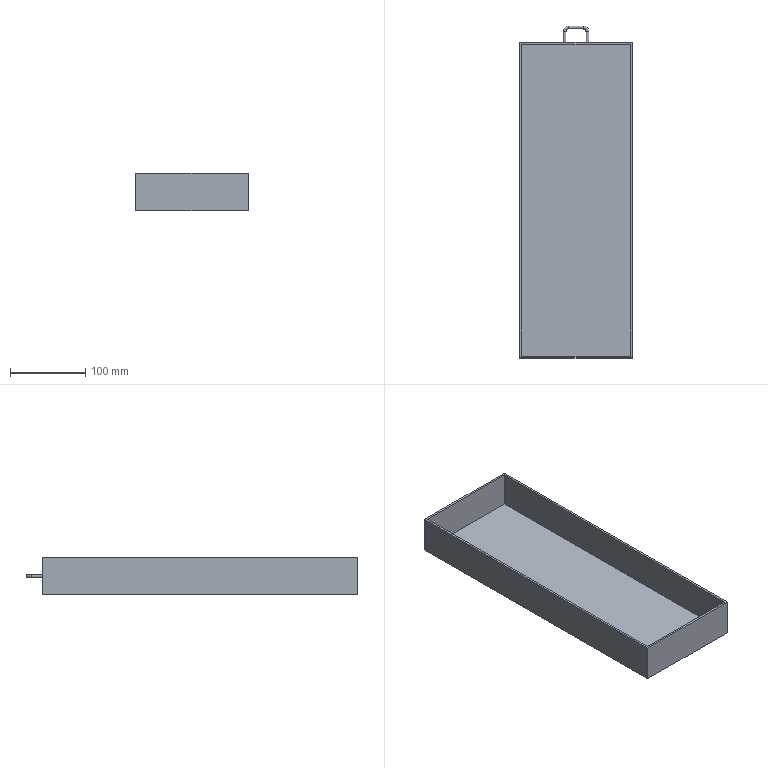Part | NX | features solid 2 | 1 solid | 16 faces | box 150 x 442 x 50 mm | volume 292513 mm3 | plane 11 | cylinder 3 | torus 2 | commonest cylinder face diameters 4 x3
STEP:
#1=CARTESIAN_POINT('',(697.,375.,-348.));
#2=VERTEX_POINT('',#1);
#3=CARTESIAN_POINT('',(697.,375.,-350.));
#4=DIRECTION('',(0.,1.,0.));
#5=DIRECTION('',(0.,0.,1.));
#6=AXIS2_PLACEMENT_3D('',#3,#4,#5);
#7=CIRCLE('',#6,2.);
#8=EDGE_CURVE('',#2,#2,#7,.T.);
#9=ORIENTED_EDGE('',*,*,#8,.F.);
#10=EDGE_LOOP('',(#9));
#11=FACE_BOUND('',#10,.T.);
#12=CARTESIAN_POINT('',(637.,375.,-375.));
#13=VERTEX_POINT('',#12);
#14=CARTESIAN_POINT('',(787.,375.,-375.));
#15=VERTEX_POINT('',#14);
#16=CARTESIAN_POINT('',(637.,375.,-375.));
#17=DIRECTION('',(1.,0.,0.));
#18=VECTOR('',#17,1000.);
#19=LINE('',#16,#18);
#20=EDGE_CURVE('',#13,#15,#19,.T.);
#21=ORIENTED_EDGE('',*,*,#20,.F.);
#22=CARTESIAN_POINT('',(637.,375.,-325.));
#23=VERTEX_POINT('',#22);
#24=CARTESIAN_POINT('',(637.,375.,-325.));
#25=DIRECTION('',(0.,0.,-1.));
#26=VECTOR('',#25,1000.);
#27=LINE('',#24,#26);
#28=EDGE_CURVE('',#23,#13,#27,.T.);
#29=ORIENTED_EDGE('',*,*,#28,.F.);
#30=CARTESIAN_POINT('',(787.,375.,-325.));
#31=VERTEX_POINT('',#30);
#32=CARTESIAN_POINT('',(637.,375.,-325.));
#33=DIRECTION('',(1.,0.,0.));
#34=VECTOR('',#33,1000.);
#35=LINE('',#32,#34);
#36=EDGE_CURVE('',#23,#31,#35,.T.);
#37=ORIENTED_EDGE('',*,*,#36,.T.);
#38=CARTESIAN_POINT('',(787.,375.,-325.));
#39=DIRECTION('',(0.,0.,-1.));
#40=VECTOR('',#39,1000.);
#41=LINE('',#38,#40);
#42=EDGE_CURVE('',#31,#15,#41,.T.);
#43=ORIENTED_EDGE('',*,*,#42,.T.);
#44=EDGE_LOOP('',(#21,#29,#37,#43));
#45=FACE_BOUND('',#44,.T.);
#46=CARTESIAN_POINT('',(727.,375.,-348.));
#47=VERTEX_POINT('',#46);
#48=CARTESIAN_POINT('',(727.,375.,-350.));
#49=DIRECTION('',(0.,1.,0.));
#50=DIRECTION('',(0.,0.,1.));
#51=AXIS2_PLACEMENT_3D('',#48,#49,#50);
#52=CIRCLE('',#51,2.);
#53=EDGE_CURVE('',#47,#47,#52,.T.);
#54=ORIENTED_EDGE('',*,*,#53,.F.);
#55=EDGE_LOOP('',(#54));
#56=FACE_BOUND('',#55,.T.);
#57=CARTESIAN_POINT('',(637.,375.,-325.));
#58=DIRECTION('',(0.,1.,0.));
#59=DIRECTION('',(0.,0.,1.));
#60=AXIS2_PLACEMENT_3D('',#57,#58,#59);
#61=PLANE('',#60);
#62=ADVANCED_FACE('',(#11,#45,#56),#61,.T.);
#63=CARTESIAN_POINT('',(784.5,372.5,-372.5));
#64=VERTEX_POINT('',#63);
#65=CARTESIAN_POINT('',(784.5,-42.5,-372.5));
#66=VERTEX_POINT('',#65);
#67=CARTESIAN_POINT('',(784.5,372.5,-372.5));
#68=DIRECTION('',(0.,-1.,0.));
#69=VECTOR('',#68,1000.);
#70=LINE('',#67,#69);
#71=EDGE_CURVE('',#64,#66,#70,.T.);
#72=ORIENTED_EDGE('',*,*,#71,.F.);
#73=CARTESIAN_POINT('',(639.5,372.5,-372.5));
#74=VERTEX_POINT('',#73);
#75=CARTESIAN_POINT('',(639.5,372.5,-372.5));
#76=DIRECTION('',(1.,0.,0.));
#77=VECTOR('',#76,1000.);
#78=LINE('',#75,#77);
#79=EDGE_CURVE('',#74,#64,#78,.T.);
#80=ORIENTED_EDGE('',*,*,#79,.F.);
#81=CARTESIAN_POINT('',(639.5,-42.5,-372.5));
#82=VERTEX_POINT('',#81);
#83=CARTESIAN_POINT('',(639.5,182.5,-372.5));
#84=DIRECTION('',(0.,1.,0.));
#85=VECTOR('',#84,1000.);
#86=LINE('',#83,#85);
#87=EDGE_CURVE('',#82,#74,#86,.T.);
#88=ORIENTED_EDGE('',*,*,#87,.F.);
#89=CARTESIAN_POINT('',(637.,-42.5,-372.5));
#90=DIRECTION('',(-1.,0.,0.));
#91=VECTOR('',#90,1000.);
#92=LINE('',#89,#91);
#93=EDGE_CURVE('',#66,#82,#92,.T.);
#94=ORIENTED_EDGE('',*,*,#93,.F.);
#95=EDGE_LOOP('',(#72,#80,#88,#94));
#96=FACE_BOUND('',#95,.T.);
#97=CARTESIAN_POINT('',(784.5,182.5,-372.5));
#98=DIRECTION('',(0.,0.,-1.));
#99=DIRECTION('',(-1.,0.,0.));
#100=AXIS2_PLACEMENT_3D('',#97,#98,#99);
#101=PLANE('',#100);
#102=ADVANCED_FACE('',(#96),#101,.F.);
#103=CARTESIAN_POINT('',(787.,-45.,-375.));
#104=VERTEX_POINT('',#103);
#105=CARTESIAN_POINT('',(637.,-45.,-375.));
#106=VERTEX_POINT('',#105);
#107=CARTESIAN_POINT('',(784.5,-45.,-375.));
#108=DIRECTION('',(-1.,0.,0.));
#109=VECTOR('',#108,1000.);
#110=LINE('',#107,#109);
#111=EDGE_CURVE('',#104,#106,#110,.T.);
#112=ORIENTED_EDGE('',*,*,#111,.T.);
#113=CARTESIAN_POINT('',(637.,372.5,-375.));
#114=DIRECTION('',(0.,1.,0.));
#115=VECTOR('',#114,1000.);
#116=LINE('',#113,#115);
#117=EDGE_CURVE('',#106,#13,#116,.T.);
#118=ORIENTED_EDGE('',*,*,#117,.T.);
#119=ORIENTED_EDGE('',*,*,#20,.T.);
#120=CARTESIAN_POINT('',(787.,375.,-375.));
#121=DIRECTION('',(0.,-1.,0.));
#122=VECTOR('',#121,1000.);
#123=LINE('',#120,#122);
#124=EDGE_CURVE('',#15,#104,#123,.T.);
#125=ORIENTED_EDGE('',*,*,#124,.T.);
#126=EDGE_LOOP('',(#112,#118,#119,#125));
#127=FACE_BOUND('',#126,.T.);
#128=CARTESIAN_POINT('',(784.5,182.5,-375.));
#129=DIRECTION('',(0.,0.,-1.));
#130=DIRECTION('',(-1.,0.,0.));
#131=AXIS2_PLACEMENT_3D('',#128,#129,#130);
#132=PLANE('',#131);
#133=ADVANCED_FACE('',(#127),#132,.T.);
#134=CARTESIAN_POINT('',(784.5,372.5,-325.));
#135=VERTEX_POINT('',#134);
#136=CARTESIAN_POINT('',(784.5,372.5,-325.));
#137=DIRECTION('',(0.,0.,-1.));
#138=VECTOR('',#137,1000.);
#139=LINE('',#136,#138);
#140=EDGE_CURVE('',#135,#64,#139,.T.);
#141=ORIENTED_EDGE('',*,*,#140,.F.);
#142=CARTESIAN_POINT('',(639.5,372.5,-325.));
#143=VERTEX_POINT('',#142);
#144=CARTESIAN_POINT('',(787.,372.5,-325.));
#145=DIRECTION('',(-1.,0.,0.));
#146=VECTOR('',#145,1000.);
#147=LINE('',#144,#146);
#148=EDGE_CURVE('',#135,#143,#147,.T.);
#149=ORIENTED_EDGE('',*,*,#148,.T.);
#150=CARTESIAN_POINT('',(639.5,372.5,-325.));
#151=DIRECTION('',(0.,0.,-1.));
#152=VECTOR('',#151,1000.);
#153=LINE('',#150,#152);
#154=EDGE_CURVE('',#143,#74,#153,.T.);
#155=ORIENTED_EDGE('',*,*,#154,.T.);
#156=ORIENTED_EDGE('',*,*,#79,.T.);
#157=EDGE_LOOP('',(#141,#149,#155,#156));
#158=FACE_BOUND('',#157,.T.);
#159=CARTESIAN_POINT('',(787.,372.5,-325.));
#160=DIRECTION('',(0.,-1.,0.));
#161=DIRECTION('',(0.,0.,-1.));
#162=AXIS2_PLACEMENT_3D('',#159,#160,#161);
#163=PLANE('',#162);
#164=ADVANCED_FACE('',(#158),#163,.T.);
#165=ORIENTED_EDGE('',*,*,#124,.F.);
#166=ORIENTED_EDGE('',*,*,#42,.F.);
#167=CARTESIAN_POINT('',(787.,-45.,-325.));
#168=VERTEX_POINT('',#167);
#169=CARTESIAN_POINT('',(787.,375.,-325.));
#170=DIRECTION('',(0.,-1.,0.));
#171=VECTOR('',#170,1000.);
#172=LINE('',#169,#171);
#173=EDGE_CURVE('',#31,#168,#172,.T.);
#174=ORIENTED_EDGE('',*,*,#173,.T.);
#175=CARTESIAN_POINT('',(787.,-45.,-325.));
#176=DIRECTION('',(0.,0.,-1.));
#177=VECTOR('',#176,1000.);
#178=LINE('',#175,#177);
#179=EDGE_CURVE('',#168,#104,#178,.T.);
#180=ORIENTED_EDGE('',*,*,#179,.T.);
#181=EDGE_LOOP('',(#165,#166,#174,#180));
#182=FACE_BOUND('',#181,.T.);
#183=CARTESIAN_POINT('',(787.,375.,-325.));
#184=DIRECTION('',(1.,0.,0.));
#185=DIRECTION('',(0.,0.,-1.));
#186=AXIS2_PLACEMENT_3D('',#183,#184,#185);
#187=PLANE('',#186);
#188=ADVANCED_FACE('',(#182),#187,.T.);
#189=ORIENTED_EDGE('',*,*,#117,.F.);
#190=CARTESIAN_POINT('',(637.,-45.,-325.));
#191=VERTEX_POINT('',#190);
#192=CARTESIAN_POINT('',(637.,-45.,-325.));
#193=DIRECTION('',(0.,0.,-1.));
#194=VECTOR('',#193,1000.);
#195=LINE('',#192,#194);
#196=EDGE_CURVE('',#191,#106,#195,.T.);
#197=ORIENTED_EDGE('',*,*,#196,.F.);
#198=CARTESIAN_POINT('',(637.,372.5,-325.));
#199=DIRECTION('',(0.,1.,0.));
#200=VECTOR('',#199,1000.);
#201=LINE('',#198,#200);
#202=EDGE_CURVE('',#191,#23,#201,.T.);
#203=ORIENTED_EDGE('',*,*,#202,.T.);
#204=ORIENTED_EDGE('',*,*,#28,.T.);
#205=EDGE_LOOP('',(#189,#197,#203,#204));
#206=FACE_BOUND('',#205,.T.);
#207=CARTESIAN_POINT('',(637.,372.5,-325.));
#208=DIRECTION('',(-1.,0.,0.));
#209=DIRECTION('',(0.,0.,1.));
#210=AXIS2_PLACEMENT_3D('',#207,#208,#209);
#211=PLANE('',#210);
#212=ADVANCED_FACE('',(#206),#211,.T.);
#213=ORIENTED_EDGE('',*,*,#148,.F.);
#214=CARTESIAN_POINT('',(784.5,-42.5,-325.));
#215=VERTEX_POINT('',#214);
#216=CARTESIAN_POINT('',(784.5,182.5,-325.));
#217=DIRECTION('',(0.,1.,0.));
#218=VECTOR('',#217,1000.);
#219=LINE('',#216,#218);
#220=EDGE_CURVE('',#215,#135,#219,.T.);
#221=ORIENTED_EDGE('',*,*,#220,.F.);
#222=CARTESIAN_POINT('',(639.5,-42.5,-325.));
#223=VERTEX_POINT('',#222);
#224=CARTESIAN_POINT('',(787.,-42.5,-325.));
#225=DIRECTION('',(1.,0.,0.));
#226=VECTOR('',#225,1000.);
#227=LINE('',#224,#226);
#228=EDGE_CURVE('',#223,#215,#227,.T.);
#229=ORIENTED_EDGE('',*,*,#228,.F.);
#230=CARTESIAN_POINT('',(639.5,372.5,-325.));
#231=DIRECTION('',(0.,-1.,0.));
#232=VECTOR('',#231,1000.);
#233=LINE('',#230,#232);
#234=EDGE_CURVE('',#143,#223,#233,.T.);
#235=ORIENTED_EDGE('',*,*,#234,.F.);
#236=EDGE_LOOP('',(#213,#221,#229,#235));
#237=FACE_BOUND('',#236,.T.);
#238=ORIENTED_EDGE('',*,*,#173,.F.);
#239=ORIENTED_EDGE('',*,*,#36,.F.);
#240=ORIENTED_EDGE('',*,*,#202,.F.);
#241=CARTESIAN_POINT('',(787.,-45.,-325.));
#242=DIRECTION('',(-1.,0.,0.));
#243=VECTOR('',#242,1000.);
#244=LINE('',#241,#243);
#245=EDGE_CURVE('',#168,#191,#244,.T.);
#246=ORIENTED_EDGE('',*,*,#245,.F.);
#247=EDGE_LOOP('',(#238,#239,#240,#246));
#248=FACE_BOUND('',#247,.T.);
#249=CARTESIAN_POINT('',(787.,372.5,-325.));
#250=DIRECTION('',(0.,0.,-1.));
#251=DIRECTION('',(-1.,0.,0.));
#252=AXIS2_PLACEMENT_3D('',#249,#250,#251);
#253=PLANE('',#252);
#254=ADVANCED_FACE('',(#237,#248),#253,.F.);
#255=CARTESIAN_POINT('',(784.5,-42.5,-325.));
#256=DIRECTION('',(0.,0.,-1.));
#257=VECTOR('',#256,1000.);
#258=LINE('',#255,#257);
#259=EDGE_CURVE('',#215,#66,#258,.T.);
#260=ORIENTED_EDGE('',*,*,#259,.T.);
#261=ORIENTED_EDGE('',*,*,#93,.T.);
#262=CARTESIAN_POINT('',(639.5,-42.5,-325.));
#263=DIRECTION('',(0.,0.,-1.));
#264=VECTOR('',#263,1000.);
#265=LINE('',#262,#264);
#266=EDGE_CURVE('',#223,#82,#265,.T.);
#267=ORIENTED_EDGE('',*,*,#266,.F.);
#268=ORIENTED_EDGE('',*,*,#228,.T.);
#269=EDGE_LOOP('',(#260,#261,#267,#268));
#270=FACE_BOUND('',#269,.T.);
#271=CARTESIAN_POINT('',(637.,-42.5,-325.));
#272=DIRECTION('',(0.,1.,0.));
#273=DIRECTION('',(0.,0.,1.));
#274=AXIS2_PLACEMENT_3D('',#271,#272,#273);
#275=PLANE('',#274);
#276=ADVANCED_FACE('',(#270),#275,.T.);
#277=ORIENTED_EDGE('',*,*,#111,.F.);
#278=ORIENTED_EDGE('',*,*,#179,.F.);
#279=ORIENTED_EDGE('',*,*,#245,.T.);
#280=ORIENTED_EDGE('',*,*,#196,.T.);
#281=EDGE_LOOP('',(#277,#278,#279,#280));
#282=FACE_BOUND('',#281,.T.);
#283=CARTESIAN_POINT('',(787.,-45.,-325.));
#284=DIRECTION('',(0.,-1.,0.));
#285=DIRECTION('',(0.,0.,-1.));
#286=AXIS2_PLACEMENT_3D('',#283,#284,#285);
#287=PLANE('',#286);
#288=ADVANCED_FACE('',(#282),#287,.T.);
#289=ORIENTED_EDGE('',*,*,#87,.T.);
#290=ORIENTED_EDGE('',*,*,#154,.F.);
#291=ORIENTED_EDGE('',*,*,#234,.T.);
#292=ORIENTED_EDGE('',*,*,#266,.T.);
#293=EDGE_LOOP('',(#289,#290,#291,#292));
#294=FACE_BOUND('',#293,.T.);
#295=CARTESIAN_POINT('',(639.5,372.5,-325.));
#296=DIRECTION('',(1.,0.,0.));
#297=DIRECTION('',(0.,0.,-1.));
#298=AXIS2_PLACEMENT_3D('',#295,#296,#297);
#299=PLANE('',#298);
#300=ADVANCED_FACE('',(#294),#299,.T.);
#301=ORIENTED_EDGE('',*,*,#71,.T.);
#302=ORIENTED_EDGE('',*,*,#259,.F.);
#303=ORIENTED_EDGE('',*,*,#220,.T.);
#304=ORIENTED_EDGE('',*,*,#140,.T.);
#305=EDGE_LOOP('',(#301,#302,#303,#304));
#306=FACE_BOUND('',#305,.T.);
#307=CARTESIAN_POINT('',(784.5,182.5,-325.));
#308=DIRECTION('',(-1.,0.,0.));
#309=DIRECTION('',(0.,0.,1.));
#310=AXIS2_PLACEMENT_3D('',#307,#308,#309);
#311=PLANE('',#310);
#312=ADVANCED_FACE('',(#306),#311,.T.);
#313=CARTESIAN_POINT('',(697.,390.,-348.));
#314=VERTEX_POINT('',#313);
#315=CARTESIAN_POINT('',(697.,390.,-350.));
#316=DIRECTION('',(0.,-1.,0.));
#317=DIRECTION('',(0.,0.,1.));
#318=AXIS2_PLACEMENT_3D('',#315,#316,#317);
#319=CIRCLE('',#318,2.);
#320=EDGE_CURVE('',#314,#314,#319,.T.);
#321=ORIENTED_EDGE('',*,*,#320,.T.);
#322=EDGE_LOOP('',(#321));
#323=FACE_BOUND('',#322,.T.);
#324=ORIENTED_EDGE('',*,*,#8,.T.);
#325=EDGE_LOOP('',(#324));
#326=FACE_BOUND('',#325,.T.);
#327=CARTESIAN_POINT('',(697.,390.,-350.));
#328=DIRECTION('',(0.,-1.,0.));
#329=DIRECTION('',(0.,0.,-1.));
#330=AXIS2_PLACEMENT_3D('',#327,#328,#329);
#331=CYLINDRICAL_SURFACE('',#330,2.);
#332=ADVANCED_FACE('',(#323,#326),#331,.T.);
#333=CARTESIAN_POINT('',(702.,395.,-348.));
#334=VERTEX_POINT('',#333);
#335=CARTESIAN_POINT('',(702.,395.,-350.));
#336=DIRECTION('',(-1.,0.,0.));
#337=DIRECTION('',(0.,0.,1.));
#338=AXIS2_PLACEMENT_3D('',#335,#336,#337);
#339=CIRCLE('',#338,2.);
#340=EDGE_CURVE('',#334,#334,#339,.T.);
#341=ORIENTED_EDGE('',*,*,#340,.T.);
#342=EDGE_LOOP('',(#341));
#343=FACE_BOUND('',#342,.T.);
#344=ORIENTED_EDGE('',*,*,#320,.F.);
#345=EDGE_LOOP('',(#344));
#346=FACE_BOUND('',#345,.T.);
#347=CARTESIAN_POINT('',(702.,390.,-350.));
#348=DIRECTION('',(0.,0.,1.));
#349=DIRECTION('',(1.,0.,0.));
#350=AXIS2_PLACEMENT_3D('',#347,#348,#349);
#351=TOROIDAL_SURFACE('',#350,5.,2.);
#352=ADVANCED_FACE('',(#343,#346),#351,.T.);
#353=CARTESIAN_POINT('',(722.,395.,-348.));
#354=VERTEX_POINT('',#353);
#355=CARTESIAN_POINT('',(722.,395.,-350.));
#356=DIRECTION('',(-1.,0.,0.));
#357=DIRECTION('',(0.,0.,1.));
#358=AXIS2_PLACEMENT_3D('',#355,#356,#357);
#359=CIRCLE('',#358,2.);
#360=EDGE_CURVE('',#354,#354,#359,.T.);
#361=ORIENTED_EDGE('',*,*,#360,.T.);
#362=EDGE_LOOP('',(#361));
#363=FACE_BOUND('',#362,.T.);
#364=ORIENTED_EDGE('',*,*,#340,.F.);
#365=EDGE_LOOP('',(#364));
#366=FACE_BOUND('',#365,.T.);
#367=CARTESIAN_POINT('',(722.,395.,-350.));
#368=DIRECTION('',(-1.,0.,0.));
#369=DIRECTION('',(0.,0.,1.));
#370=AXIS2_PLACEMENT_3D('',#367,#368,#369);
#371=CYLINDRICAL_SURFACE('',#370,2.);
#372=ADVANCED_FACE('',(#363,#366),#371,.T.);
#373=CARTESIAN_POINT('',(727.,390.,-348.));
#374=VERTEX_POINT('',#373);
#375=CARTESIAN_POINT('',(727.,390.,-350.));
#376=DIRECTION('',(0.,1.,0.));
#377=DIRECTION('',(0.,0.,1.));
#378=AXIS2_PLACEMENT_3D('',#375,#376,#377);
#379=CIRCLE('',#378,2.);
#380=EDGE_CURVE('',#374,#374,#379,.T.);
#381=ORIENTED_EDGE('',*,*,#380,.T.);
#382=EDGE_LOOP('',(#381));
#383=FACE_BOUND('',#382,.T.);
#384=ORIENTED_EDGE('',*,*,#360,.F.);
#385=EDGE_LOOP('',(#384));
#386=FACE_BOUND('',#385,.T.);
#387=CARTESIAN_POINT('',(722.,390.,-350.));
#388=DIRECTION('',(0.,0.,1.));
#389=DIRECTION('',(1.,0.,0.));
#390=AXIS2_PLACEMENT_3D('',#387,#388,#389);
#391=TOROIDAL_SURFACE('',#390,5.,2.);
#392=ADVANCED_FACE('',(#383,#386),#391,.T.);
#393=ORIENTED_EDGE('',*,*,#380,.F.);
#394=EDGE_LOOP('',(#393));
#395=FACE_BOUND('',#394,.T.);
#396=ORIENTED_EDGE('',*,*,#53,.T.);
#397=EDGE_LOOP('',(#396));
#398=FACE_BOUND('',#397,.T.);
#399=CARTESIAN_POINT('',(727.,390.,-350.));
#400=DIRECTION('',(0.,-1.,0.));
#401=DIRECTION('',(0.,0.,-1.));
#402=AXIS2_PLACEMENT_3D('',#399,#400,#401);
#403=CYLINDRICAL_SURFACE('',#402,2.);
#404=ADVANCED_FACE('',(#395,#398),#403,.T.);
#405=CLOSED_SHELL('',(#62,#102,#133,#164,#188,#212,#254,#276,#288,#300,#312,#332,#352,#372,#392,#404));
#406=MANIFOLD_SOLID_BREP('',#405);
#407=(LENGTH_UNIT()NAMED_UNIT(*)SI_UNIT(.MILLI.,.METRE.));
#408=UNCERTAINTY_MEASURE_WITH_UNIT(LENGTH_MEASURE(0.00001),#407,'','');
#409=(NAMED_UNIT(*)PLANE_ANGLE_UNIT()SI_UNIT($,.RADIAN.));
#410=(NAMED_UNIT(*)SI_UNIT($,.STERADIAN.)SOLID_ANGLE_UNIT());
#411=(GEOMETRIC_REPRESENTATION_CONTEXT(3)GLOBAL_UNCERTAINTY_ASSIGNED_CONTEXT((#408))GLOBAL_UNIT_ASSIGNED_CONTEXT((#407,#409,#410))REPRESENTATION_CONTEXT('',''));
#412=ADVANCED_BREP_SHAPE_REPRESENTATION('',(#406),#411);